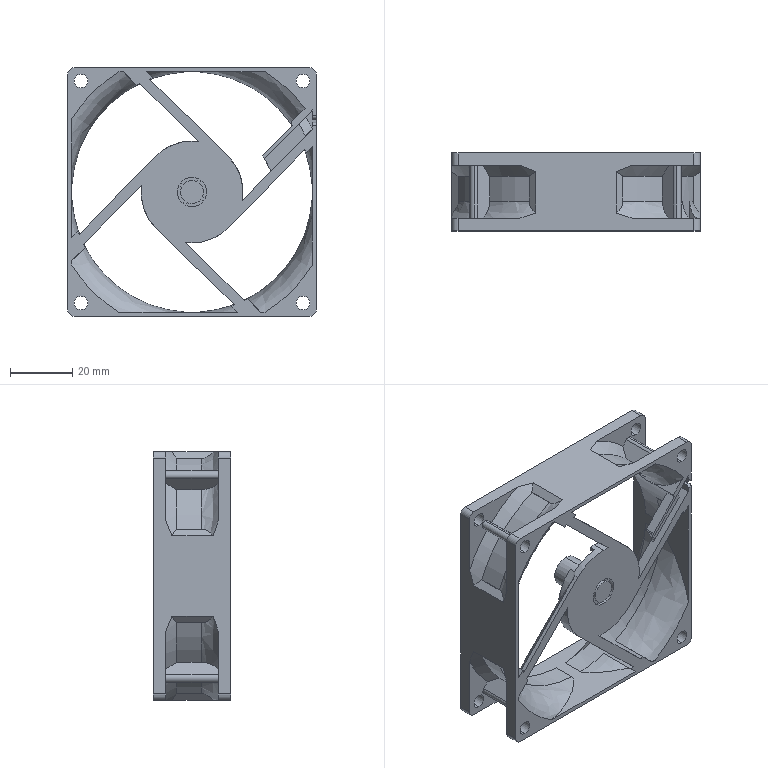Part | STEP file | 8025R_9_1.stp | 1 solid | 237 faces | box 80 x 25 x 80 mm | volume 22585 mm3 | plane 120 | cylinder 88 | spline 17 | cone 12 | commonest cylinder face diameters 4 x24 4.4 x16 81.5 x8 2.8 x6 7.4 x5 9.4 x5